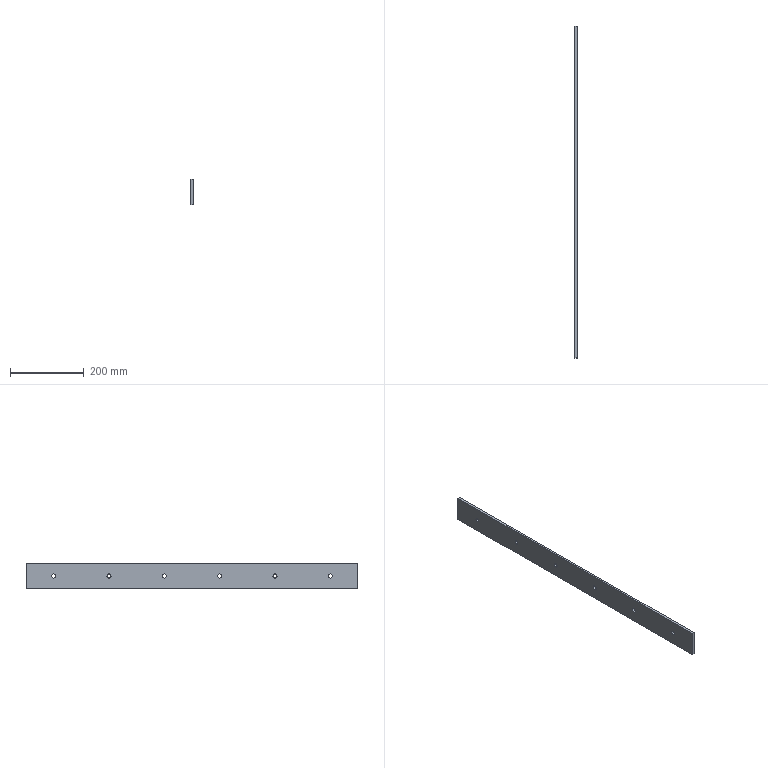Part | NX | features DATUM_CSYS 2, EXTRUDE 1, SKETCH 1 | 1 solid | 12 faces | box 6 x 900 x 70 mm | volume 374579 mm3 | plane 6 | cylinder 6 | commonest cylinder face diameters 11 x6
STEP:
#1=CARTESIAN_POINT('',(0.,0.,70.));
#2=VERTEX_POINT('',#1);
#3=CARTESIAN_POINT('',(0.,0.,0.));
#4=VERTEX_POINT('',#3);
#5=CARTESIAN_POINT('',(0.,0.,70.));
#6=DIRECTION('',(0.,0.,-1.));
#7=VECTOR('',#6,1000.);
#8=LINE('',#5,#7);
#9=EDGE_CURVE('',#2,#4,#8,.T.);
#10=ORIENTED_EDGE('',*,*,#9,.T.);
#11=CARTESIAN_POINT('',(6.,0.,0.));
#12=VERTEX_POINT('',#11);
#13=CARTESIAN_POINT('',(6.,0.,0.));
#14=DIRECTION('',(-1.,0.,0.));
#15=VECTOR('',#14,1000.);
#16=LINE('',#13,#15);
#17=EDGE_CURVE('',#12,#4,#16,.T.);
#18=ORIENTED_EDGE('',*,*,#17,.F.);
#19=CARTESIAN_POINT('',(6.,0.,70.));
#20=VERTEX_POINT('',#19);
#21=CARTESIAN_POINT('',(6.,0.,70.));
#22=DIRECTION('',(0.,0.,-1.));
#23=VECTOR('',#22,1000.);
#24=LINE('',#21,#23);
#25=EDGE_CURVE('',#20,#12,#24,.T.);
#26=ORIENTED_EDGE('',*,*,#25,.F.);
#27=CARTESIAN_POINT('',(6.,0.,70.));
#28=DIRECTION('',(-1.,0.,0.));
#29=VECTOR('',#28,1000.);
#30=LINE('',#27,#29);
#31=EDGE_CURVE('',#20,#2,#30,.T.);
#32=ORIENTED_EDGE('',*,*,#31,.T.);
#33=EDGE_LOOP('',(#10,#18,#26,#32));
#34=FACE_BOUND('',#33,.T.);
#35=CARTESIAN_POINT('',(6.,0.,70.));
#36=DIRECTION('',(0.,1.,0.));
#37=DIRECTION('',(0.,0.,1.));
#38=AXIS2_PLACEMENT_3D('',#35,#36,#37);
#39=PLANE('',#38);
#40=ADVANCED_FACE('',(#34),#39,.F.);
#41=CARTESIAN_POINT('',(0.,900.,0.));
#42=VERTEX_POINT('',#41);
#43=CARTESIAN_POINT('',(0.,0.,0.));
#44=DIRECTION('',(0.,1.,0.));
#45=VECTOR('',#44,1000.);
#46=LINE('',#43,#45);
#47=EDGE_CURVE('',#4,#42,#46,.T.);
#48=ORIENTED_EDGE('',*,*,#47,.T.);
#49=CARTESIAN_POINT('',(6.,900.,0.));
#50=VERTEX_POINT('',#49);
#51=CARTESIAN_POINT('',(6.,900.,0.));
#52=DIRECTION('',(-1.,0.,0.));
#53=VECTOR('',#52,1000.);
#54=LINE('',#51,#53);
#55=EDGE_CURVE('',#50,#42,#54,.T.);
#56=ORIENTED_EDGE('',*,*,#55,.F.);
#57=CARTESIAN_POINT('',(6.,0.,0.));
#58=DIRECTION('',(0.,1.,0.));
#59=VECTOR('',#58,1000.);
#60=LINE('',#57,#59);
#61=EDGE_CURVE('',#12,#50,#60,.T.);
#62=ORIENTED_EDGE('',*,*,#61,.F.);
#63=ORIENTED_EDGE('',*,*,#17,.T.);
#64=EDGE_LOOP('',(#48,#56,#62,#63));
#65=FACE_BOUND('',#64,.T.);
#66=CARTESIAN_POINT('',(6.,0.,0.));
#67=DIRECTION('',(0.,0.,1.));
#68=DIRECTION('',(1.,0.,0.));
#69=AXIS2_PLACEMENT_3D('',#66,#67,#68);
#70=PLANE('',#69);
#71=ADVANCED_FACE('',(#65),#70,.F.);
#72=CARTESIAN_POINT('',(0.,900.,70.));
#73=VERTEX_POINT('',#72);
#74=CARTESIAN_POINT('',(0.,900.,0.));
#75=DIRECTION('',(0.,0.,1.));
#76=VECTOR('',#75,1000.);
#77=LINE('',#74,#76);
#78=EDGE_CURVE('',#42,#73,#77,.T.);
#79=ORIENTED_EDGE('',*,*,#78,.T.);
#80=CARTESIAN_POINT('',(6.,900.,70.));
#81=VERTEX_POINT('',#80);
#82=CARTESIAN_POINT('',(6.,900.,70.));
#83=DIRECTION('',(-1.,0.,0.));
#84=VECTOR('',#83,1000.);
#85=LINE('',#82,#84);
#86=EDGE_CURVE('',#81,#73,#85,.T.);
#87=ORIENTED_EDGE('',*,*,#86,.F.);
#88=CARTESIAN_POINT('',(6.,900.,0.));
#89=DIRECTION('',(0.,0.,1.));
#90=VECTOR('',#89,1000.);
#91=LINE('',#88,#90);
#92=EDGE_CURVE('',#50,#81,#91,.T.);
#93=ORIENTED_EDGE('',*,*,#92,.F.);
#94=ORIENTED_EDGE('',*,*,#55,.T.);
#95=EDGE_LOOP('',(#79,#87,#93,#94));
#96=FACE_BOUND('',#95,.T.);
#97=CARTESIAN_POINT('',(6.,900.,0.));
#98=DIRECTION('',(0.,-1.,0.));
#99=DIRECTION('',(0.,0.,-1.));
#100=AXIS2_PLACEMENT_3D('',#97,#98,#99);
#101=PLANE('',#100);
#102=ADVANCED_FACE('',(#96),#101,.F.);
#103=CARTESIAN_POINT('',(6.,680.5,35.));
#104=VERTEX_POINT('',#103);
#105=CARTESIAN_POINT('',(6.,675.,35.));
#106=DIRECTION('',(1.,0.,0.));
#107=DIRECTION('',(0.,1.,0.));
#108=AXIS2_PLACEMENT_3D('',#105,#106,#107);
#109=CIRCLE('',#108,5.5);
#110=EDGE_CURVE('',#104,#104,#109,.T.);
#111=ORIENTED_EDGE('',*,*,#110,.T.);
#112=EDGE_LOOP('',(#111));
#113=FACE_BOUND('',#112,.T.);
#114=CARTESIAN_POINT('',(0.,680.5,35.));
#115=VERTEX_POINT('',#114);
#116=CARTESIAN_POINT('',(0.,675.,35.));
#117=DIRECTION('',(1.,0.,0.));
#118=DIRECTION('',(0.,1.,0.));
#119=AXIS2_PLACEMENT_3D('',#116,#117,#118);
#120=CIRCLE('',#119,5.5);
#121=EDGE_CURVE('',#115,#115,#120,.T.);
#122=ORIENTED_EDGE('',*,*,#121,.F.);
#123=EDGE_LOOP('',(#122));
#124=FACE_BOUND('',#123,.T.);
#125=CARTESIAN_POINT('',(6.,675.,35.));
#126=DIRECTION('',(-1.,0.,0.));
#127=DIRECTION('',(0.,0.,1.));
#128=AXIS2_PLACEMENT_3D('',#125,#126,#127);
#129=CYLINDRICAL_SURFACE('',#128,5.5);
#130=ADVANCED_FACE('',(#113,#124),#129,.F.);
#131=CARTESIAN_POINT('',(6.,530.5,35.));
#132=VERTEX_POINT('',#131);
#133=CARTESIAN_POINT('',(6.,525.,35.));
#134=DIRECTION('',(1.,0.,0.));
#135=DIRECTION('',(0.,1.,0.));
#136=AXIS2_PLACEMENT_3D('',#133,#134,#135);
#137=CIRCLE('',#136,5.5);
#138=EDGE_CURVE('',#132,#132,#137,.T.);
#139=ORIENTED_EDGE('',*,*,#138,.T.);
#140=EDGE_LOOP('',(#139));
#141=FACE_BOUND('',#140,.T.);
#142=CARTESIAN_POINT('',(0.,530.5,35.));
#143=VERTEX_POINT('',#142);
#144=CARTESIAN_POINT('',(0.,525.,35.));
#145=DIRECTION('',(1.,0.,0.));
#146=DIRECTION('',(0.,1.,0.));
#147=AXIS2_PLACEMENT_3D('',#144,#145,#146);
#148=CIRCLE('',#147,5.5);
#149=EDGE_CURVE('',#143,#143,#148,.T.);
#150=ORIENTED_EDGE('',*,*,#149,.F.);
#151=EDGE_LOOP('',(#150));
#152=FACE_BOUND('',#151,.T.);
#153=CARTESIAN_POINT('',(6.,525.,35.));
#154=DIRECTION('',(-1.,0.,0.));
#155=DIRECTION('',(0.,0.,1.));
#156=AXIS2_PLACEMENT_3D('',#153,#154,#155);
#157=CYLINDRICAL_SURFACE('',#156,5.5);
#158=ADVANCED_FACE('',(#141,#152),#157,.F.);
#159=CARTESIAN_POINT('',(6.,380.5,35.));
#160=VERTEX_POINT('',#159);
#161=CARTESIAN_POINT('',(6.,375.,35.));
#162=DIRECTION('',(1.,0.,0.));
#163=DIRECTION('',(0.,1.,0.));
#164=AXIS2_PLACEMENT_3D('',#161,#162,#163);
#165=CIRCLE('',#164,5.5);
#166=EDGE_CURVE('',#160,#160,#165,.T.);
#167=ORIENTED_EDGE('',*,*,#166,.T.);
#168=EDGE_LOOP('',(#167));
#169=FACE_BOUND('',#168,.T.);
#170=CARTESIAN_POINT('',(0.,380.5,35.));
#171=VERTEX_POINT('',#170);
#172=CARTESIAN_POINT('',(0.,375.,35.));
#173=DIRECTION('',(1.,0.,0.));
#174=DIRECTION('',(0.,1.,0.));
#175=AXIS2_PLACEMENT_3D('',#172,#173,#174);
#176=CIRCLE('',#175,5.5);
#177=EDGE_CURVE('',#171,#171,#176,.T.);
#178=ORIENTED_EDGE('',*,*,#177,.F.);
#179=EDGE_LOOP('',(#178));
#180=FACE_BOUND('',#179,.T.);
#181=CARTESIAN_POINT('',(6.,375.,35.));
#182=DIRECTION('',(-1.,0.,0.));
#183=DIRECTION('',(0.,0.,1.));
#184=AXIS2_PLACEMENT_3D('',#181,#182,#183);
#185=CYLINDRICAL_SURFACE('',#184,5.5);
#186=ADVANCED_FACE('',(#169,#180),#185,.F.);
#187=CARTESIAN_POINT('',(6.,230.5,35.));
#188=VERTEX_POINT('',#187);
#189=CARTESIAN_POINT('',(6.,225.,35.));
#190=DIRECTION('',(1.,0.,0.));
#191=DIRECTION('',(0.,1.,0.));
#192=AXIS2_PLACEMENT_3D('',#189,#190,#191);
#193=CIRCLE('',#192,5.5);
#194=EDGE_CURVE('',#188,#188,#193,.T.);
#195=ORIENTED_EDGE('',*,*,#194,.T.);
#196=EDGE_LOOP('',(#195));
#197=FACE_BOUND('',#196,.T.);
#198=CARTESIAN_POINT('',(0.,230.5,35.));
#199=VERTEX_POINT('',#198);
#200=CARTESIAN_POINT('',(0.,225.,35.));
#201=DIRECTION('',(1.,0.,0.));
#202=DIRECTION('',(0.,1.,0.));
#203=AXIS2_PLACEMENT_3D('',#200,#201,#202);
#204=CIRCLE('',#203,5.5);
#205=EDGE_CURVE('',#199,#199,#204,.T.);
#206=ORIENTED_EDGE('',*,*,#205,.F.);
#207=EDGE_LOOP('',(#206));
#208=FACE_BOUND('',#207,.T.);
#209=CARTESIAN_POINT('',(6.,225.,35.));
#210=DIRECTION('',(-1.,0.,0.));
#211=DIRECTION('',(0.,0.,1.));
#212=AXIS2_PLACEMENT_3D('',#209,#210,#211);
#213=CYLINDRICAL_SURFACE('',#212,5.5);
#214=ADVANCED_FACE('',(#197,#208),#213,.F.);
#215=CARTESIAN_POINT('',(6.,80.5,35.));
#216=VERTEX_POINT('',#215);
#217=CARTESIAN_POINT('',(6.,75.,35.));
#218=DIRECTION('',(1.,0.,0.));
#219=DIRECTION('',(0.,1.,0.));
#220=AXIS2_PLACEMENT_3D('',#217,#218,#219);
#221=CIRCLE('',#220,5.5);
#222=EDGE_CURVE('',#216,#216,#221,.T.);
#223=ORIENTED_EDGE('',*,*,#222,.T.);
#224=EDGE_LOOP('',(#223));
#225=FACE_BOUND('',#224,.T.);
#226=CARTESIAN_POINT('',(0.,80.5,35.));
#227=VERTEX_POINT('',#226);
#228=CARTESIAN_POINT('',(0.,75.,35.));
#229=DIRECTION('',(1.,0.,0.));
#230=DIRECTION('',(0.,1.,0.));
#231=AXIS2_PLACEMENT_3D('',#228,#229,#230);
#232=CIRCLE('',#231,5.5);
#233=EDGE_CURVE('',#227,#227,#232,.T.);
#234=ORIENTED_EDGE('',*,*,#233,.F.);
#235=EDGE_LOOP('',(#234));
#236=FACE_BOUND('',#235,.T.);
#237=CARTESIAN_POINT('',(6.,75.,35.));
#238=DIRECTION('',(-1.,0.,0.));
#239=DIRECTION('',(0.,0.,1.));
#240=AXIS2_PLACEMENT_3D('',#237,#238,#239);
#241=CYLINDRICAL_SURFACE('',#240,5.5);
#242=ADVANCED_FACE('',(#225,#236),#241,.F.);
#243=CARTESIAN_POINT('',(0.,900.,70.));
#244=DIRECTION('',(0.,-1.,0.));
#245=VECTOR('',#244,1000.);
#246=LINE('',#243,#245);
#247=EDGE_CURVE('',#73,#2,#246,.T.);
#248=ORIENTED_EDGE('',*,*,#247,.T.);
#249=ORIENTED_EDGE('',*,*,#31,.F.);
#250=CARTESIAN_POINT('',(6.,900.,70.));
#251=DIRECTION('',(0.,-1.,0.));
#252=VECTOR('',#251,1000.);
#253=LINE('',#250,#252);
#254=EDGE_CURVE('',#81,#20,#253,.T.);
#255=ORIENTED_EDGE('',*,*,#254,.F.);
#256=ORIENTED_EDGE('',*,*,#86,.T.);
#257=EDGE_LOOP('',(#248,#249,#255,#256));
#258=FACE_BOUND('',#257,.T.);
#259=CARTESIAN_POINT('',(6.,900.,70.));
#260=DIRECTION('',(0.,0.,-1.));
#261=DIRECTION('',(-1.,0.,0.));
#262=AXIS2_PLACEMENT_3D('',#259,#260,#261);
#263=PLANE('',#262);
#264=ADVANCED_FACE('',(#258),#263,.F.);
#265=CARTESIAN_POINT('',(6.,830.5,35.));
#266=VERTEX_POINT('',#265);
#267=CARTESIAN_POINT('',(6.,825.,35.));
#268=DIRECTION('',(1.,0.,0.));
#269=DIRECTION('',(0.,1.,0.));
#270=AXIS2_PLACEMENT_3D('',#267,#268,#269);
#271=CIRCLE('',#270,5.5);
#272=EDGE_CURVE('',#266,#266,#271,.T.);
#273=ORIENTED_EDGE('',*,*,#272,.T.);
#274=EDGE_LOOP('',(#273));
#275=FACE_BOUND('',#274,.T.);
#276=CARTESIAN_POINT('',(0.,830.5,35.));
#277=VERTEX_POINT('',#276);
#278=CARTESIAN_POINT('',(0.,825.,35.));
#279=DIRECTION('',(1.,0.,0.));
#280=DIRECTION('',(0.,1.,0.));
#281=AXIS2_PLACEMENT_3D('',#278,#279,#280);
#282=CIRCLE('',#281,5.5);
#283=EDGE_CURVE('',#277,#277,#282,.T.);
#284=ORIENTED_EDGE('',*,*,#283,.F.);
#285=EDGE_LOOP('',(#284));
#286=FACE_BOUND('',#285,.T.);
#287=CARTESIAN_POINT('',(6.,825.,35.));
#288=DIRECTION('',(-1.,0.,0.));
#289=DIRECTION('',(0.,0.,1.));
#290=AXIS2_PLACEMENT_3D('',#287,#288,#289);
#291=CYLINDRICAL_SURFACE('',#290,5.5);
#292=ADVANCED_FACE('',(#275,#286),#291,.F.);
#293=ORIENTED_EDGE('',*,*,#25,.T.);
#294=ORIENTED_EDGE('',*,*,#61,.T.);
#295=ORIENTED_EDGE('',*,*,#92,.T.);
#296=ORIENTED_EDGE('',*,*,#254,.T.);
#297=EDGE_LOOP('',(#293,#294,#295,#296));
#298=FACE_BOUND('',#297,.T.);
#299=ORIENTED_EDGE('',*,*,#222,.F.);
#300=EDGE_LOOP('',(#299));
#301=FACE_BOUND('',#300,.T.);
#302=ORIENTED_EDGE('',*,*,#194,.F.);
#303=EDGE_LOOP('',(#302));
#304=FACE_BOUND('',#303,.T.);
#305=ORIENTED_EDGE('',*,*,#166,.F.);
#306=EDGE_LOOP('',(#305));
#307=FACE_BOUND('',#306,.T.);
#308=ORIENTED_EDGE('',*,*,#138,.F.);
#309=EDGE_LOOP('',(#308));
#310=FACE_BOUND('',#309,.T.);
#311=ORIENTED_EDGE('',*,*,#110,.F.);
#312=EDGE_LOOP('',(#311));
#313=FACE_BOUND('',#312,.T.);
#314=ORIENTED_EDGE('',*,*,#272,.F.);
#315=EDGE_LOOP('',(#314));
#316=FACE_BOUND('',#315,.T.);
#317=CARTESIAN_POINT('',(6.,75.,35.));
#318=DIRECTION('',(1.,0.,0.));
#319=DIRECTION('',(0.,0.,-1.));
#320=AXIS2_PLACEMENT_3D('',#317,#318,#319);
#321=PLANE('',#320);
#322=ADVANCED_FACE('',(#298,#301,#304,#307,#310,#313,#316),#321,.T.);
#323=ORIENTED_EDGE('',*,*,#9,.F.);
#324=ORIENTED_EDGE('',*,*,#247,.F.);
#325=ORIENTED_EDGE('',*,*,#78,.F.);
#326=ORIENTED_EDGE('',*,*,#47,.F.);
#327=EDGE_LOOP('',(#323,#324,#325,#326));
#328=FACE_BOUND('',#327,.T.);
#329=ORIENTED_EDGE('',*,*,#233,.T.);
#330=EDGE_LOOP('',(#329));
#331=FACE_BOUND('',#330,.T.);
#332=ORIENTED_EDGE('',*,*,#205,.T.);
#333=EDGE_LOOP('',(#332));
#334=FACE_BOUND('',#333,.T.);
#335=ORIENTED_EDGE('',*,*,#177,.T.);
#336=EDGE_LOOP('',(#335));
#337=FACE_BOUND('',#336,.T.);
#338=ORIENTED_EDGE('',*,*,#149,.T.);
#339=EDGE_LOOP('',(#338));
#340=FACE_BOUND('',#339,.T.);
#341=ORIENTED_EDGE('',*,*,#121,.T.);
#342=EDGE_LOOP('',(#341));
#343=FACE_BOUND('',#342,.T.);
#344=ORIENTED_EDGE('',*,*,#283,.T.);
#345=EDGE_LOOP('',(#344));
#346=FACE_BOUND('',#345,.T.);
#347=CARTESIAN_POINT('',(0.,75.,35.));
#348=DIRECTION('',(1.,0.,0.));
#349=DIRECTION('',(0.,0.,-1.));
#350=AXIS2_PLACEMENT_3D('',#347,#348,#349);
#351=PLANE('',#350);
#352=ADVANCED_FACE('',(#328,#331,#334,#337,#340,#343,#346),#351,.F.);
#353=CLOSED_SHELL('',(#40,#71,#102,#130,#158,#186,#214,#242,#264,#292,#322,#352));
#354=MANIFOLD_SOLID_BREP('',#353);
#355=(LENGTH_UNIT()NAMED_UNIT(*)SI_UNIT(.MILLI.,.METRE.));
#356=UNCERTAINTY_MEASURE_WITH_UNIT(LENGTH_MEASURE(0.00001),#355,'','');
#357=(NAMED_UNIT(*)PLANE_ANGLE_UNIT()SI_UNIT($,.RADIAN.));
#358=(NAMED_UNIT(*)SI_UNIT($,.STERADIAN.)SOLID_ANGLE_UNIT());
#359=(GEOMETRIC_REPRESENTATION_CONTEXT(3)GLOBAL_UNCERTAINTY_ASSIGNED_CONTEXT((#356))GLOBAL_UNIT_ASSIGNED_CONTEXT((#355,#357,#358))REPRESENTATION_CONTEXT('',''));
#360=ADVANCED_BREP_SHAPE_REPRESENTATION('',(#354),#359);